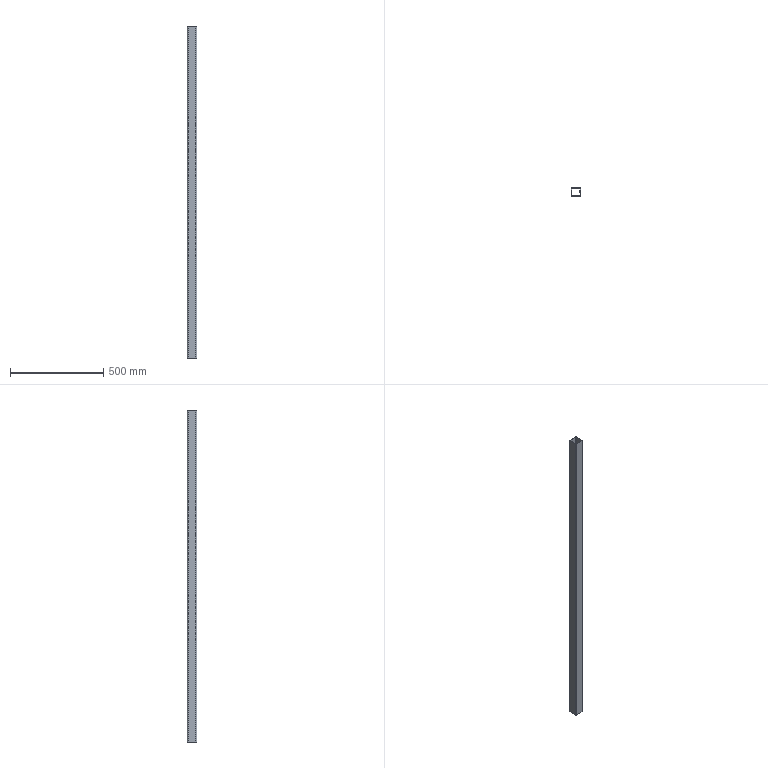Part | SolidWorks | features BaseBody 1 | 1 solid | 69 faces | box 50 x 50 x 1776 mm | volume 972714 mm3 | cylinder 50 | plane 19 | commonest cylinder face diameters 13 x30 6.5 x8 2 x4 8 x4 6 x2 18 x2